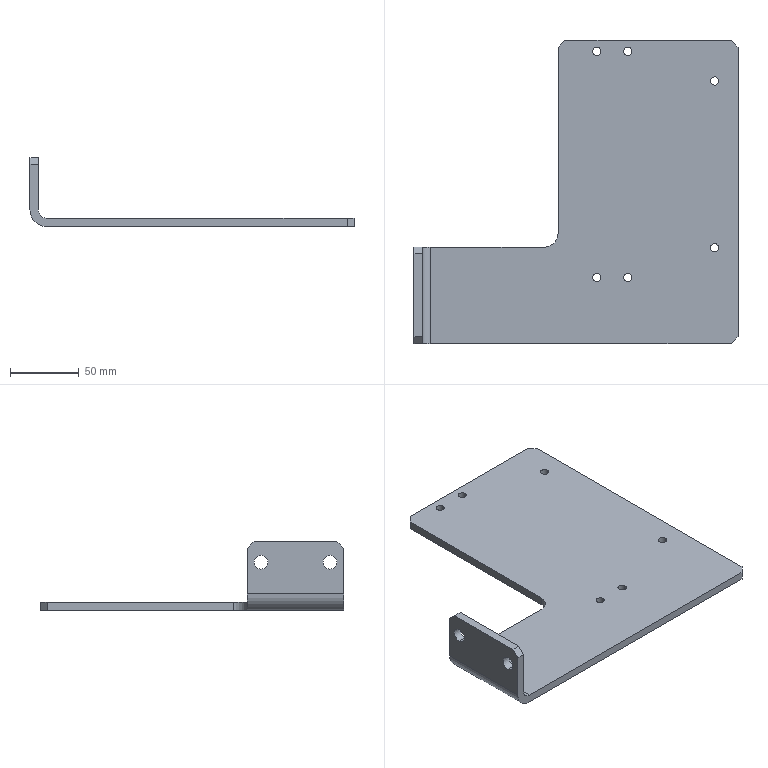Part | STEP file | [02]-13 | 1 solid | 34 faces | box 235 x 220 x 50 mm | volume 230801 mm3 | cylinder 19 | plane 15 | commonest cylinder face diameters 6 x12 10 x4 12 x1 20 x1 24 x1